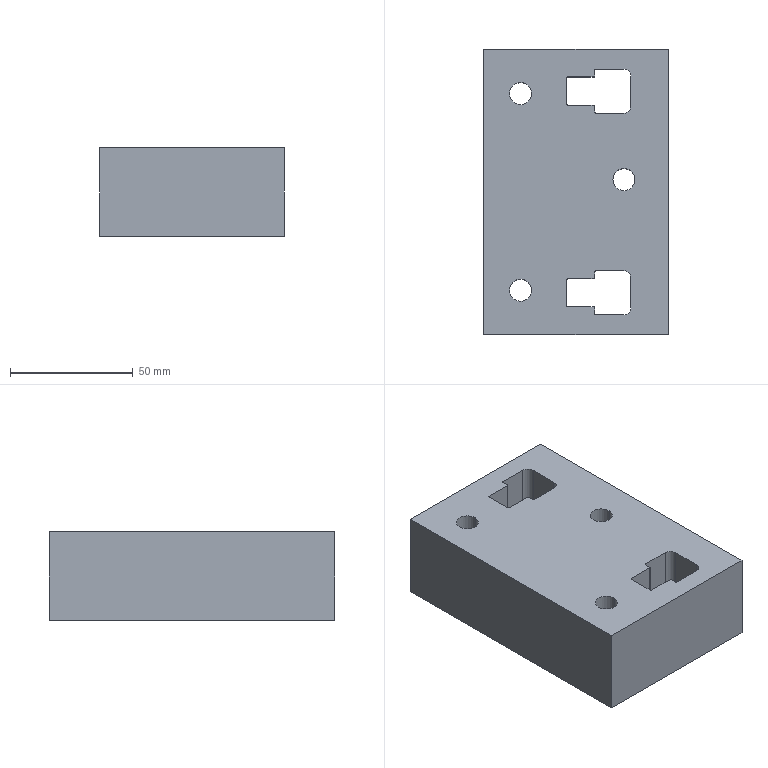Part | 1 solid | 61 faces | box 75 x 116 x 36 mm | volume 273588 mm3 | cylinder 32 | plane 25 | cone 4 | commonest cylinder face diameters 1 x8 9 x6 14 x6 0.6 x4 6 x4 8 x4